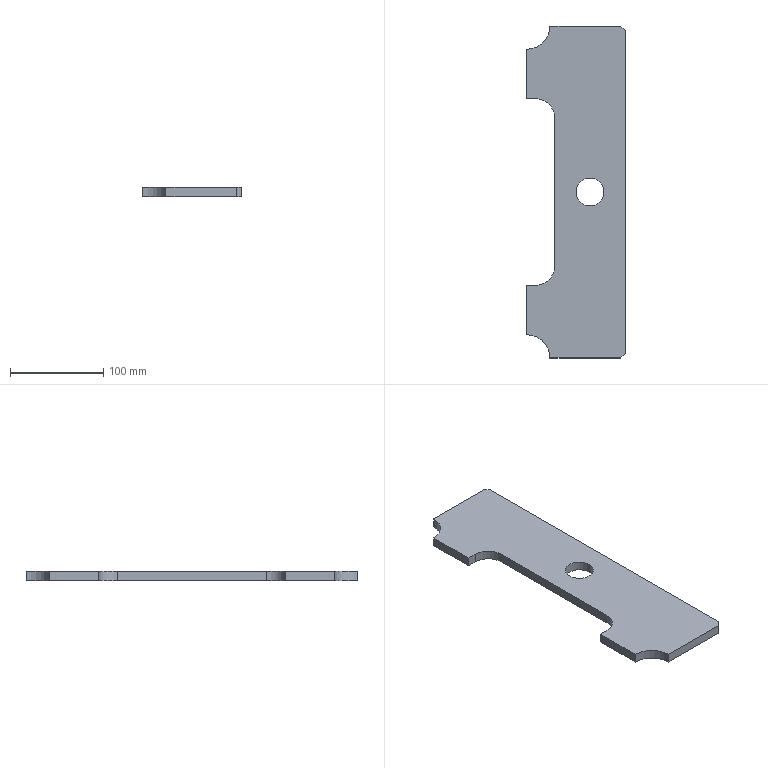Part | STEP file | VD-SYL0380DJ1006_1_1-14_VD-SYL0 | 1 solid | 18 faces | box 106 x 356 x 10 mm | volume 301941 mm3 | plane 12 | cylinder 6 | commonest cylinder face diameters 30 x2 40 x2 50 x2
STEP:
#1=CARTESIAN_POINT('',(0.,0.,10.));
#2=VERTEX_POINT('',#1);
#3=CARTESIAN_POINT('',(30.,0.,10.));
#4=VERTEX_POINT('',#3);
#5=CARTESIAN_POINT('',(15.,0.,10.));
#6=DIRECTION('',(0.,0.,-1.));
#7=DIRECTION('',(-1.,0.,0.));
#8=AXIS2_PLACEMENT_3D('',#5,#6,#7);
#9=CIRCLE('',#8,15.);
#10=EDGE_CURVE('',#2,#4,#9,.T.);
#11=ORIENTED_EDGE('',*,*,#10,.F.);
#12=CARTESIAN_POINT('',(0.,0.,0.));
#13=VERTEX_POINT('',#12);
#14=CARTESIAN_POINT('',(0.,0.,0.));
#15=DIRECTION('',(0.,0.,1.));
#16=VECTOR('',#15,1000.);
#17=LINE('',#14,#16);
#18=EDGE_CURVE('',#13,#2,#17,.T.);
#19=ORIENTED_EDGE('',*,*,#18,.F.);
#20=CARTESIAN_POINT('',(30.,0.,0.));
#21=VERTEX_POINT('',#20);
#22=CARTESIAN_POINT('',(15.,0.,0.));
#23=DIRECTION('',(0.,0.,1.));
#24=DIRECTION('',(1.,0.,0.));
#25=AXIS2_PLACEMENT_3D('',#22,#23,#24);
#26=CIRCLE('',#25,15.);
#27=EDGE_CURVE('',#21,#13,#26,.T.);
#28=ORIENTED_EDGE('',*,*,#27,.F.);
#29=CARTESIAN_POINT('',(30.,0.,0.));
#30=DIRECTION('',(0.,0.,1.));
#31=VECTOR('',#30,1000.);
#32=LINE('',#29,#31);
#33=EDGE_CURVE('',#21,#4,#32,.T.);
#34=ORIENTED_EDGE('',*,*,#33,.T.);
#35=EDGE_LOOP('',(#11,#19,#28,#34));
#36=FACE_OUTER_BOUND('',#35,.T.);
#37=CARTESIAN_POINT('',(15.,0.,5.));
#38=DIRECTION('',(0.,0.,-1.));
#39=DIRECTION('',(-1.,0.,0.));
#40=AXIS2_PLACEMENT_3D('',#37,#38,#39);
#41=CYLINDRICAL_SURFACE('',#40,15.);
#42=ADVANCED_FACE('',(#36),#41,.F.);
#43=ORIENTED_EDGE('',*,*,#33,.F.);
#44=CARTESIAN_POINT('',(15.,0.,0.));
#45=DIRECTION('',(0.,0.,1.));
#46=DIRECTION('',(-1.,0.,0.));
#47=AXIS2_PLACEMENT_3D('',#44,#45,#46);
#48=CIRCLE('',#47,15.);
#49=EDGE_CURVE('',#13,#21,#48,.T.);
#50=ORIENTED_EDGE('',*,*,#49,.F.);
#51=ORIENTED_EDGE('',*,*,#18,.T.);
#52=CARTESIAN_POINT('',(15.,0.,10.));
#53=DIRECTION('',(0.,0.,-1.));
#54=DIRECTION('',(1.,0.,0.));
#55=AXIS2_PLACEMENT_3D('',#52,#53,#54);
#56=CIRCLE('',#55,15.);
#57=EDGE_CURVE('',#4,#2,#56,.T.);
#58=ORIENTED_EDGE('',*,*,#57,.F.);
#59=EDGE_LOOP('',(#43,#50,#51,#58));
#60=FACE_OUTER_BOUND('',#59,.T.);
#61=CARTESIAN_POINT('',(15.,0.,5.));
#62=DIRECTION('',(0.,0.,-1.));
#63=DIRECTION('',(-1.,0.,0.));
#64=AXIS2_PLACEMENT_3D('',#61,#62,#63);
#65=CYLINDRICAL_SURFACE('',#64,15.);
#66=ADVANCED_FACE('',(#60),#65,.F.);
#67=CARTESIAN_POINT('',(-53.,-153.,10.));
#68=VERTEX_POINT('',#67);
#69=CARTESIAN_POINT('',(-53.,-153.,0.));
#70=VERTEX_POINT('',#69);
#71=CARTESIAN_POINT('',(-53.,-153.,10.));
#72=DIRECTION('',(0.,0.,-1.));
#73=VECTOR('',#72,1000.);
#74=LINE('',#71,#73);
#75=EDGE_CURVE('',#68,#70,#74,.T.);
#76=ORIENTED_EDGE('',*,*,#75,.T.);
#77=CARTESIAN_POINT('',(-28.,-178.,0.));
#78=VERTEX_POINT('',#77);
#79=CARTESIAN_POINT('',(-53.,-178.,0.));
#80=DIRECTION('',(0.,0.,1.));
#81=DIRECTION('',(1.,0.,0.));
#82=AXIS2_PLACEMENT_3D('',#79,#80,#81);
#83=CIRCLE('',#82,25.);
#84=EDGE_CURVE('',#78,#70,#83,.T.);
#85=ORIENTED_EDGE('',*,*,#84,.F.);
#86=CARTESIAN_POINT('',(-28.,-178.,10.));
#87=VERTEX_POINT('',#86);
#88=CARTESIAN_POINT('',(-28.,-178.,0.));
#89=DIRECTION('',(0.,0.,1.));
#90=VECTOR('',#89,1000.);
#91=LINE('',#88,#90);
#92=EDGE_CURVE('',#78,#87,#91,.T.);
#93=ORIENTED_EDGE('',*,*,#92,.T.);
#94=CARTESIAN_POINT('',(-53.,-178.,10.));
#95=DIRECTION('',(0.,0.,-1.));
#96=DIRECTION('',(0.,1.,0.));
#97=AXIS2_PLACEMENT_3D('',#94,#95,#96);
#98=CIRCLE('',#97,25.);
#99=EDGE_CURVE('',#68,#87,#98,.T.);
#100=ORIENTED_EDGE('',*,*,#99,.F.);
#101=EDGE_LOOP('',(#76,#85,#93,#100));
#102=FACE_OUTER_BOUND('',#101,.T.);
#103=CARTESIAN_POINT('',(-53.,-178.,5.));
#104=DIRECTION('',(0.,0.,-1.));
#105=DIRECTION('',(-1.,0.,0.));
#106=AXIS2_PLACEMENT_3D('',#103,#104,#105);
#107=CYLINDRICAL_SURFACE('',#106,25.);
#108=ADVANCED_FACE('',(#102),#107,.F.);
#109=CARTESIAN_POINT('',(-43.,-100.,0.));
#110=VERTEX_POINT('',#109);
#111=CARTESIAN_POINT('',(-23.,-80.,0.));
#112=VERTEX_POINT('',#111);
#113=CARTESIAN_POINT('',(-43.,-80.,0.));
#114=DIRECTION('',(0.,0.,1.));
#115=DIRECTION('',(0.,-1.,0.));
#116=AXIS2_PLACEMENT_3D('',#113,#114,#115);
#117=CIRCLE('',#116,20.);
#118=EDGE_CURVE('',#110,#112,#117,.T.);
#119=ORIENTED_EDGE('',*,*,#118,.F.);
#120=CARTESIAN_POINT('',(-43.,-100.,10.));
#121=VERTEX_POINT('',#120);
#122=CARTESIAN_POINT('',(-43.,-100.,0.));
#123=DIRECTION('',(0.,0.,1.));
#124=VECTOR('',#123,1000.);
#125=LINE('',#122,#124);
#126=EDGE_CURVE('',#110,#121,#125,.T.);
#127=ORIENTED_EDGE('',*,*,#126,.T.);
#128=CARTESIAN_POINT('',(-23.,-80.,10.));
#129=VERTEX_POINT('',#128);
#130=CARTESIAN_POINT('',(-43.,-80.,10.));
#131=DIRECTION('',(0.,0.,-1.));
#132=DIRECTION('',(1.,0.,0.));
#133=AXIS2_PLACEMENT_3D('',#130,#131,#132);
#134=CIRCLE('',#133,20.);
#135=EDGE_CURVE('',#129,#121,#134,.T.);
#136=ORIENTED_EDGE('',*,*,#135,.F.);
#137=CARTESIAN_POINT('',(-23.,-80.,10.));
#138=DIRECTION('',(0.,0.,-1.));
#139=VECTOR('',#138,1000.);
#140=LINE('',#137,#139);
#141=EDGE_CURVE('',#129,#112,#140,.T.);
#142=ORIENTED_EDGE('',*,*,#141,.T.);
#143=EDGE_LOOP('',(#119,#127,#136,#142));
#144=FACE_OUTER_BOUND('',#143,.T.);
#145=CARTESIAN_POINT('',(-43.,-80.,-25.06));
#146=DIRECTION('',(0.,0.,1.));
#147=DIRECTION('',(1.,0.,0.));
#148=AXIS2_PLACEMENT_3D('',#145,#146,#147);
#149=CYLINDRICAL_SURFACE('',#148,20.);
#150=ADVANCED_FACE('',(#144),#149,.F.);
#151=CARTESIAN_POINT('',(-23.,80.,0.));
#152=VERTEX_POINT('',#151);
#153=CARTESIAN_POINT('',(-23.,80.,0.));
#154=DIRECTION('',(0.,-1.,0.));
#155=VECTOR('',#154,1000.);
#156=LINE('',#153,#155);
#157=EDGE_CURVE('',#152,#112,#156,.T.);
#158=ORIENTED_EDGE('',*,*,#157,.T.);
#159=ORIENTED_EDGE('',*,*,#141,.F.);
#160=CARTESIAN_POINT('',(-23.,80.,10.));
#161=VERTEX_POINT('',#160);
#162=CARTESIAN_POINT('',(-23.,-80.,10.));
#163=DIRECTION('',(0.,1.,0.));
#164=VECTOR('',#163,1000.);
#165=LINE('',#162,#164);
#166=EDGE_CURVE('',#129,#161,#165,.T.);
#167=ORIENTED_EDGE('',*,*,#166,.T.);
#168=CARTESIAN_POINT('',(-23.,80.,0.));
#169=DIRECTION('',(0.,0.,1.));
#170=VECTOR('',#169,1000.);
#171=LINE('',#168,#170);
#172=EDGE_CURVE('',#152,#161,#171,.T.);
#173=ORIENTED_EDGE('',*,*,#172,.F.);
#174=EDGE_LOOP('',(#158,#159,#167,#173));
#175=FACE_OUTER_BOUND('',#174,.T.);
#176=CARTESIAN_POINT('',(-23.,0.,5.));
#177=DIRECTION('',(1.,0.,0.));
#178=DIRECTION('',(0.,1.,0.));
#179=AXIS2_PLACEMENT_3D('',#176,#177,#178);
#180=PLANE('',#179);
#181=ADVANCED_FACE('',(#175),#180,.F.);
#182=CARTESIAN_POINT('',(-43.,100.,0.));
#183=VERTEX_POINT('',#182);
#184=CARTESIAN_POINT('',(-43.,80.,0.));
#185=DIRECTION('',(0.,0.,1.));
#186=DIRECTION('',(1.,0.,0.));
#187=AXIS2_PLACEMENT_3D('',#184,#185,#186);
#188=CIRCLE('',#187,20.);
#189=EDGE_CURVE('',#152,#183,#188,.T.);
#190=ORIENTED_EDGE('',*,*,#189,.F.);
#191=ORIENTED_EDGE('',*,*,#172,.T.);
#192=CARTESIAN_POINT('',(-43.,100.,10.));
#193=VERTEX_POINT('',#192);
#194=CARTESIAN_POINT('',(-43.,80.,10.));
#195=DIRECTION('',(0.,0.,-1.));
#196=DIRECTION('',(0.,1.,0.));
#197=AXIS2_PLACEMENT_3D('',#194,#195,#196);
#198=CIRCLE('',#197,20.);
#199=EDGE_CURVE('',#193,#161,#198,.T.);
#200=ORIENTED_EDGE('',*,*,#199,.F.);
#201=CARTESIAN_POINT('',(-43.,100.,10.));
#202=DIRECTION('',(0.,0.,-1.));
#203=VECTOR('',#202,1000.);
#204=LINE('',#201,#203);
#205=EDGE_CURVE('',#193,#183,#204,.T.);
#206=ORIENTED_EDGE('',*,*,#205,.T.);
#207=EDGE_LOOP('',(#190,#191,#200,#206));
#208=FACE_OUTER_BOUND('',#207,.T.);
#209=CARTESIAN_POINT('',(-43.,80.,-25.06));
#210=DIRECTION('',(0.,0.,1.));
#211=DIRECTION('',(1.,0.,0.));
#212=AXIS2_PLACEMENT_3D('',#209,#210,#211);
#213=CYLINDRICAL_SURFACE('',#212,20.);
#214=ADVANCED_FACE('',(#208),#213,.F.);
#215=CARTESIAN_POINT('',(-53.,100.,0.));
#216=VERTEX_POINT('',#215);
#217=CARTESIAN_POINT('',(-53.,100.,0.));
#218=DIRECTION('',(1.,0.,0.));
#219=VECTOR('',#218,1000.);
#220=LINE('',#217,#219);
#221=EDGE_CURVE('',#216,#183,#220,.T.);
#222=ORIENTED_EDGE('',*,*,#221,.T.);
#223=ORIENTED_EDGE('',*,*,#205,.F.);
#224=CARTESIAN_POINT('',(-53.,100.,10.));
#225=VERTEX_POINT('',#224);
#226=CARTESIAN_POINT('',(-43.,100.,10.));
#227=DIRECTION('',(-1.,0.,0.));
#228=VECTOR('',#227,1000.);
#229=LINE('',#226,#228);
#230=EDGE_CURVE('',#193,#225,#229,.T.);
#231=ORIENTED_EDGE('',*,*,#230,.T.);
#232=CARTESIAN_POINT('',(-53.,100.,10.));
#233=DIRECTION('',(0.,0.,-1.));
#234=VECTOR('',#233,1000.);
#235=LINE('',#232,#234);
#236=EDGE_CURVE('',#225,#216,#235,.T.);
#237=ORIENTED_EDGE('',*,*,#236,.T.);
#238=EDGE_LOOP('',(#222,#223,#231,#237));
#239=FACE_OUTER_BOUND('',#238,.T.);
#240=CARTESIAN_POINT('',(-38.,100.,5.));
#241=DIRECTION('',(0.,1.,0.));
#242=DIRECTION('',(1.,0.,0.));
#243=AXIS2_PLACEMENT_3D('',#240,#241,#242);
#244=PLANE('',#243);
#245=ADVANCED_FACE('',(#239),#244,.F.);
#246=CARTESIAN_POINT('',(-53.,153.,10.));
#247=VERTEX_POINT('',#246);
#248=CARTESIAN_POINT('',(-53.,100.,10.));
#249=DIRECTION('',(0.,1.,0.));
#250=VECTOR('',#249,1000.);
#251=LINE('',#248,#250);
#252=EDGE_CURVE('',#225,#247,#251,.T.);
#253=ORIENTED_EDGE('',*,*,#252,.T.);
#254=CARTESIAN_POINT('',(-53.,153.,0.));
#255=VERTEX_POINT('',#254);
#256=CARTESIAN_POINT('',(-53.,153.,0.));
#257=DIRECTION('',(0.,0.,1.));
#258=VECTOR('',#257,1000.);
#259=LINE('',#256,#258);
#260=EDGE_CURVE('',#255,#247,#259,.T.);
#261=ORIENTED_EDGE('',*,*,#260,.F.);
#262=CARTESIAN_POINT('',(-53.,153.,0.));
#263=DIRECTION('',(0.,-1.,0.));
#264=VECTOR('',#263,1000.);
#265=LINE('',#262,#264);
#266=EDGE_CURVE('',#255,#216,#265,.T.);
#267=ORIENTED_EDGE('',*,*,#266,.T.);
#268=ORIENTED_EDGE('',*,*,#236,.F.);
#269=EDGE_LOOP('',(#253,#261,#267,#268));
#270=FACE_OUTER_BOUND('',#269,.T.);
#271=CARTESIAN_POINT('',(-53.,0.,5.));
#272=DIRECTION('',(1.,0.,0.));
#273=DIRECTION('',(0.,1.,0.));
#274=AXIS2_PLACEMENT_3D('',#271,#272,#273);
#275=PLANE('',#274);
#276=ADVANCED_FACE('',(#270),#275,.F.);
#277=CARTESIAN_POINT('',(-28.,178.,10.));
#278=VERTEX_POINT('',#277);
#279=CARTESIAN_POINT('',(-28.,178.,0.));
#280=VERTEX_POINT('',#279);
#281=CARTESIAN_POINT('',(-28.,178.,10.));
#282=DIRECTION('',(0.,0.,-1.));
#283=VECTOR('',#282,1000.);
#284=LINE('',#281,#283);
#285=EDGE_CURVE('',#278,#280,#284,.T.);
#286=ORIENTED_EDGE('',*,*,#285,.T.);
#287=CARTESIAN_POINT('',(-53.,178.,0.));
#288=DIRECTION('',(0.,0.,1.));
#289=DIRECTION('',(0.,-1.,0.));
#290=AXIS2_PLACEMENT_3D('',#287,#288,#289);
#291=CIRCLE('',#290,25.);
#292=EDGE_CURVE('',#255,#280,#291,.T.);
#293=ORIENTED_EDGE('',*,*,#292,.F.);
#294=ORIENTED_EDGE('',*,*,#260,.T.);
#295=CARTESIAN_POINT('',(-53.,178.,10.));
#296=DIRECTION('',(0.,0.,-1.));
#297=DIRECTION('',(1.,0.,0.));
#298=AXIS2_PLACEMENT_3D('',#295,#296,#297);
#299=CIRCLE('',#298,25.);
#300=EDGE_CURVE('',#278,#247,#299,.T.);
#301=ORIENTED_EDGE('',*,*,#300,.F.);
#302=EDGE_LOOP('',(#286,#293,#294,#301));
#303=FACE_OUTER_BOUND('',#302,.T.);
#304=CARTESIAN_POINT('',(-53.,178.,5.));
#305=DIRECTION('',(0.,0.,-1.));
#306=DIRECTION('',(-1.,0.,0.));
#307=AXIS2_PLACEMENT_3D('',#304,#305,#306);
#308=CYLINDRICAL_SURFACE('',#307,25.);
#309=ADVANCED_FACE('',(#303),#308,.F.);
#310=ORIENTED_EDGE('',*,*,#27,.T.);
#311=ORIENTED_EDGE('',*,*,#49,.T.);
#312=EDGE_LOOP('',(#310,#311));
#313=FACE_BOUND('',#312,.T.);
#314=CARTESIAN_POINT('',(53.,-173.,0.));
#315=VERTEX_POINT('',#314);
#316=CARTESIAN_POINT('',(53.,173.,0.));
#317=VERTEX_POINT('',#316);
#318=CARTESIAN_POINT('',(53.,-173.,0.));
#319=DIRECTION('',(0.,1.,0.));
#320=VECTOR('',#319,1000.);
#321=LINE('',#318,#320);
#322=EDGE_CURVE('',#315,#317,#321,.T.);
#323=ORIENTED_EDGE('',*,*,#322,.F.);
#324=CARTESIAN_POINT('',(48.,-178.,0.));
#325=VERTEX_POINT('',#324);
#326=CARTESIAN_POINT('',(53.,-173.,0.));
#327=DIRECTION('',(-0.7071,-0.7071,0.));
#328=VECTOR('',#327,1000.);
#329=LINE('',#326,#328);
#330=EDGE_CURVE('',#315,#325,#329,.T.);
#331=ORIENTED_EDGE('',*,*,#330,.T.);
#332=CARTESIAN_POINT('',(-28.,-178.,0.));
#333=DIRECTION('',(1.,0.,0.));
#334=VECTOR('',#333,1000.);
#335=LINE('',#332,#334);
#336=EDGE_CURVE('',#78,#325,#335,.T.);
#337=ORIENTED_EDGE('',*,*,#336,.F.);
#338=ORIENTED_EDGE('',*,*,#84,.T.);
#339=CARTESIAN_POINT('',(-53.,-100.,0.));
#340=VERTEX_POINT('',#339);
#341=CARTESIAN_POINT('',(-53.,-100.,0.));
#342=DIRECTION('',(0.,-1.,0.));
#343=VECTOR('',#342,1000.);
#344=LINE('',#341,#343);
#345=EDGE_CURVE('',#340,#70,#344,.T.);
#346=ORIENTED_EDGE('',*,*,#345,.F.);
#347=CARTESIAN_POINT('',(-53.,-100.,0.));
#348=DIRECTION('',(1.,0.,0.));
#349=VECTOR('',#348,1000.);
#350=LINE('',#347,#349);
#351=EDGE_CURVE('',#340,#110,#350,.T.);
#352=ORIENTED_EDGE('',*,*,#351,.T.);
#353=ORIENTED_EDGE('',*,*,#118,.T.);
#354=ORIENTED_EDGE('',*,*,#157,.F.);
#355=ORIENTED_EDGE('',*,*,#189,.T.);
#356=ORIENTED_EDGE('',*,*,#221,.F.);
#357=ORIENTED_EDGE('',*,*,#266,.F.);
#358=ORIENTED_EDGE('',*,*,#292,.T.);
#359=CARTESIAN_POINT('',(48.,178.,0.));
#360=VERTEX_POINT('',#359);
#361=CARTESIAN_POINT('',(48.,178.,0.));
#362=DIRECTION('',(-1.,0.,0.));
#363=VECTOR('',#362,1000.);
#364=LINE('',#361,#363);
#365=EDGE_CURVE('',#360,#280,#364,.T.);
#366=ORIENTED_EDGE('',*,*,#365,.F.);
#367=CARTESIAN_POINT('',(48.,178.,0.));
#368=DIRECTION('',(0.7071,-0.7071,0.));
#369=VECTOR('',#368,1000.);
#370=LINE('',#367,#369);
#371=EDGE_CURVE('',#360,#317,#370,.T.);
#372=ORIENTED_EDGE('',*,*,#371,.T.);
#373=EDGE_LOOP('',(#323,#331,#337,#338,#346,#352,#353,#354,#355,#356,#357,#358,#366,#372));
#374=FACE_OUTER_BOUND('',#373,.T.);
#375=CARTESIAN_POINT('',(0.,0.,0.));
#376=DIRECTION('',(0.,0.,1.));
#377=DIRECTION('',(1.,0.,0.));
#378=AXIS2_PLACEMENT_3D('',#375,#376,#377);
#379=PLANE('',#378);
#380=ADVANCED_FACE('',(#313,#374),#379,.F.);
#381=CARTESIAN_POINT('',(48.,-178.,10.));
#382=VERTEX_POINT('',#381);
#383=CARTESIAN_POINT('',(48.,-178.,10.));
#384=DIRECTION('',(-1.,0.,0.));
#385=VECTOR('',#384,1000.);
#386=LINE('',#383,#385);
#387=EDGE_CURVE('',#382,#87,#386,.T.);
#388=ORIENTED_EDGE('',*,*,#387,.T.);
#389=ORIENTED_EDGE('',*,*,#92,.F.);
#390=ORIENTED_EDGE('',*,*,#336,.T.);
#391=CARTESIAN_POINT('',(48.,-178.,0.));
#392=DIRECTION('',(0.,0.,1.));
#393=VECTOR('',#392,1000.);
#394=LINE('',#391,#393);
#395=EDGE_CURVE('',#325,#382,#394,.T.);
#396=ORIENTED_EDGE('',*,*,#395,.T.);
#397=EDGE_LOOP('',(#388,#389,#390,#396));
#398=FACE_OUTER_BOUND('',#397,.T.);
#399=CARTESIAN_POINT('',(0.,-178.,5.));
#400=DIRECTION('',(0.,1.,0.));
#401=DIRECTION('',(1.,0.,0.));
#402=AXIS2_PLACEMENT_3D('',#399,#400,#401);
#403=PLANE('',#402);
#404=ADVANCED_FACE('',(#398),#403,.F.);
#405=ORIENTED_EDGE('',*,*,#330,.F.);
#406=CARTESIAN_POINT('',(53.,-173.,10.));
#407=VERTEX_POINT('',#406);
#408=CARTESIAN_POINT('',(53.,-173.,10.));
#409=DIRECTION('',(0.,0.,-1.));
#410=VECTOR('',#409,1000.);
#411=LINE('',#408,#410);
#412=EDGE_CURVE('',#407,#315,#411,.T.);
#413=ORIENTED_EDGE('',*,*,#412,.F.);
#414=CARTESIAN_POINT('',(48.,-178.,10.));
#415=DIRECTION('',(0.7071,0.7071,0.));
#416=VECTOR('',#415,1000.);
#417=LINE('',#414,#416);
#418=EDGE_CURVE('',#382,#407,#417,.T.);
#419=ORIENTED_EDGE('',*,*,#418,.F.);
#420=ORIENTED_EDGE('',*,*,#395,.F.);
#421=EDGE_LOOP('',(#405,#413,#419,#420));
#422=FACE_OUTER_BOUND('',#421,.T.);
#423=CARTESIAN_POINT('',(50.5,-175.5,5.));
#424=DIRECTION('',(0.7071,-0.7071,0.));
#425=DIRECTION('',(0.,0.,-1.));
#426=AXIS2_PLACEMENT_3D('',#423,#424,#425);
#427=PLANE('',#426);
#428=ADVANCED_FACE('',(#422),#427,.T.);
#429=ORIENTED_EDGE('',*,*,#322,.T.);
#430=CARTESIAN_POINT('',(53.,173.,10.));
#431=VERTEX_POINT('',#430);
#432=CARTESIAN_POINT('',(53.,173.,0.));
#433=DIRECTION('',(0.,0.,1.));
#434=VECTOR('',#433,1000.);
#435=LINE('',#432,#434);
#436=EDGE_CURVE('',#317,#431,#435,.T.);
#437=ORIENTED_EDGE('',*,*,#436,.T.);
#438=CARTESIAN_POINT('',(53.,173.,10.));
#439=DIRECTION('',(0.,-1.,0.));
#440=VECTOR('',#439,1000.);
#441=LINE('',#438,#440);
#442=EDGE_CURVE('',#431,#407,#441,.T.);
#443=ORIENTED_EDGE('',*,*,#442,.T.);
#444=ORIENTED_EDGE('',*,*,#412,.T.);
#445=EDGE_LOOP('',(#429,#437,#443,#444));
#446=FACE_OUTER_BOUND('',#445,.T.);
#447=CARTESIAN_POINT('',(53.,0.,5.));
#448=DIRECTION('',(-1.,0.,0.));
#449=DIRECTION('',(0.,0.,1.));
#450=AXIS2_PLACEMENT_3D('',#447,#448,#449);
#451=PLANE('',#450);
#452=ADVANCED_FACE('',(#446),#451,.F.);
#453=ORIENTED_EDGE('',*,*,#371,.F.);
#454=CARTESIAN_POINT('',(48.,178.,10.));
#455=VERTEX_POINT('',#454);
#456=CARTESIAN_POINT('',(48.,178.,10.));
#457=DIRECTION('',(0.,0.,-1.));
#458=VECTOR('',#457,1000.);
#459=LINE('',#456,#458);
#460=EDGE_CURVE('',#455,#360,#459,.T.);
#461=ORIENTED_EDGE('',*,*,#460,.F.);
#462=CARTESIAN_POINT('',(53.,173.,10.));
#463=DIRECTION('',(-0.7071,0.7071,0.));
#464=VECTOR('',#463,1000.);
#465=LINE('',#462,#464);
#466=EDGE_CURVE('',#431,#455,#465,.T.);
#467=ORIENTED_EDGE('',*,*,#466,.F.);
#468=ORIENTED_EDGE('',*,*,#436,.F.);
#469=EDGE_LOOP('',(#453,#461,#467,#468));
#470=FACE_OUTER_BOUND('',#469,.T.);
#471=CARTESIAN_POINT('',(50.5,175.5,5.));
#472=DIRECTION('',(0.7071,0.7071,0.));
#473=DIRECTION('',(0.,0.,-1.));
#474=AXIS2_PLACEMENT_3D('',#471,#472,#473);
#475=PLANE('',#474);
#476=ADVANCED_FACE('',(#470),#475,.T.);
#477=ORIENTED_EDGE('',*,*,#365,.T.);
#478=ORIENTED_EDGE('',*,*,#285,.F.);
#479=CARTESIAN_POINT('',(-28.,178.,10.));
#480=DIRECTION('',(1.,0.,0.));
#481=VECTOR('',#480,1000.);
#482=LINE('',#479,#481);
#483=EDGE_CURVE('',#278,#455,#482,.T.);
#484=ORIENTED_EDGE('',*,*,#483,.T.);
#485=ORIENTED_EDGE('',*,*,#460,.T.);
#486=EDGE_LOOP('',(#477,#478,#484,#485));
#487=FACE_OUTER_BOUND('',#486,.T.);
#488=CARTESIAN_POINT('',(0.,178.,5.));
#489=DIRECTION('',(0.,-1.,0.));
#490=DIRECTION('',(0.,0.,-1.));
#491=AXIS2_PLACEMENT_3D('',#488,#489,#490);
#492=PLANE('',#491);
#493=ADVANCED_FACE('',(#487),#492,.F.);
#494=ORIENTED_EDGE('',*,*,#57,.T.);
#495=ORIENTED_EDGE('',*,*,#10,.T.);
#496=EDGE_LOOP('',(#494,#495));
#497=FACE_BOUND('',#496,.T.);
#498=ORIENTED_EDGE('',*,*,#300,.T.);
#499=ORIENTED_EDGE('',*,*,#252,.F.);
#500=ORIENTED_EDGE('',*,*,#230,.F.);
#501=ORIENTED_EDGE('',*,*,#199,.T.);
#502=ORIENTED_EDGE('',*,*,#166,.F.);
#503=ORIENTED_EDGE('',*,*,#135,.T.);
#504=CARTESIAN_POINT('',(-53.,-100.,10.));
#505=VERTEX_POINT('',#504);
#506=CARTESIAN_POINT('',(-53.,-100.,10.));
#507=DIRECTION('',(1.,0.,0.));
#508=VECTOR('',#507,1000.);
#509=LINE('',#506,#508);
#510=EDGE_CURVE('',#505,#121,#509,.T.);
#511=ORIENTED_EDGE('',*,*,#510,.F.);
#512=CARTESIAN_POINT('',(-53.,-153.,10.));
#513=DIRECTION('',(0.,1.,0.));
#514=VECTOR('',#513,1000.);
#515=LINE('',#512,#514);
#516=EDGE_CURVE('',#68,#505,#515,.T.);
#517=ORIENTED_EDGE('',*,*,#516,.F.);
#518=ORIENTED_EDGE('',*,*,#99,.T.);
#519=ORIENTED_EDGE('',*,*,#387,.F.);
#520=ORIENTED_EDGE('',*,*,#418,.T.);
#521=ORIENTED_EDGE('',*,*,#442,.F.);
#522=ORIENTED_EDGE('',*,*,#466,.T.);
#523=ORIENTED_EDGE('',*,*,#483,.F.);
#524=EDGE_LOOP('',(#498,#499,#500,#501,#502,#503,#511,#517,#518,#519,#520,#521,#522,#523));
#525=FACE_OUTER_BOUND('',#524,.T.);
#526=CARTESIAN_POINT('',(0.,0.,10.));
#527=DIRECTION('',(0.,0.,1.));
#528=DIRECTION('',(1.,0.,0.));
#529=AXIS2_PLACEMENT_3D('',#526,#527,#528);
#530=PLANE('',#529);
#531=ADVANCED_FACE('',(#497,#525),#530,.T.);
#532=ORIENTED_EDGE('',*,*,#126,.F.);
#533=ORIENTED_EDGE('',*,*,#351,.F.);
#534=CARTESIAN_POINT('',(-53.,-100.,10.));
#535=DIRECTION('',(0.,0.,-1.));
#536=VECTOR('',#535,1000.);
#537=LINE('',#534,#536);
#538=EDGE_CURVE('',#505,#340,#537,.T.);
#539=ORIENTED_EDGE('',*,*,#538,.F.);
#540=ORIENTED_EDGE('',*,*,#510,.T.);
#541=EDGE_LOOP('',(#532,#533,#539,#540));
#542=FACE_OUTER_BOUND('',#541,.T.);
#543=CARTESIAN_POINT('',(-38.,-100.,5.));
#544=DIRECTION('',(0.,1.,0.));
#545=DIRECTION('',(1.,0.,0.));
#546=AXIS2_PLACEMENT_3D('',#543,#544,#545);
#547=PLANE('',#546);
#548=ADVANCED_FACE('',(#542),#547,.T.);
#549=ORIENTED_EDGE('',*,*,#345,.T.);
#550=ORIENTED_EDGE('',*,*,#75,.F.);
#551=ORIENTED_EDGE('',*,*,#516,.T.);
#552=ORIENTED_EDGE('',*,*,#538,.T.);
#553=EDGE_LOOP('',(#549,#550,#551,#552));
#554=FACE_OUTER_BOUND('',#553,.T.);
#555=CARTESIAN_POINT('',(-53.,0.,5.));
#556=DIRECTION('',(1.,0.,0.));
#557=DIRECTION('',(0.,1.,0.));
#558=AXIS2_PLACEMENT_3D('',#555,#556,#557);
#559=PLANE('',#558);
#560=ADVANCED_FACE('',(#554),#559,.F.);
#561=CLOSED_SHELL('',(#42,#66,#108,#150,#181,#214,#245,#276,#309,#380,#404,#428,#452,#476,#493,#531,#548,#560));
#562=MANIFOLD_SOLID_BREP('',#561);
#563=CARTESIAN_POINT('',(0.,0.,0.));
#564=DIRECTION('',(0.,0.,1.));
#565=DIRECTION('',(1.,0.,0.));
#566=AXIS2_PLACEMENT_3D('',#563,#564,#565);
#567=(LENGTH_UNIT()NAMED_UNIT(*)SI_UNIT(.MILLI.,.METRE.));
#568=UNCERTAINTY_MEASURE_WITH_UNIT(LENGTH_MEASURE(0.00001),#567,'','');
#569=(NAMED_UNIT(*)PLANE_ANGLE_UNIT()SI_UNIT($,.RADIAN.));
#570=(NAMED_UNIT(*)SI_UNIT($,.STERADIAN.)SOLID_ANGLE_UNIT());
#571=(GEOMETRIC_REPRESENTATION_CONTEXT(3)GLOBAL_UNCERTAINTY_ASSIGNED_CONTEXT((#568))GLOBAL_UNIT_ASSIGNED_CONTEXT((#567,#569,#570))REPRESENTATION_CONTEXT('',''));
#572=ADVANCED_BREP_SHAPE_REPRESENTATION('',(#562,#566),#571);